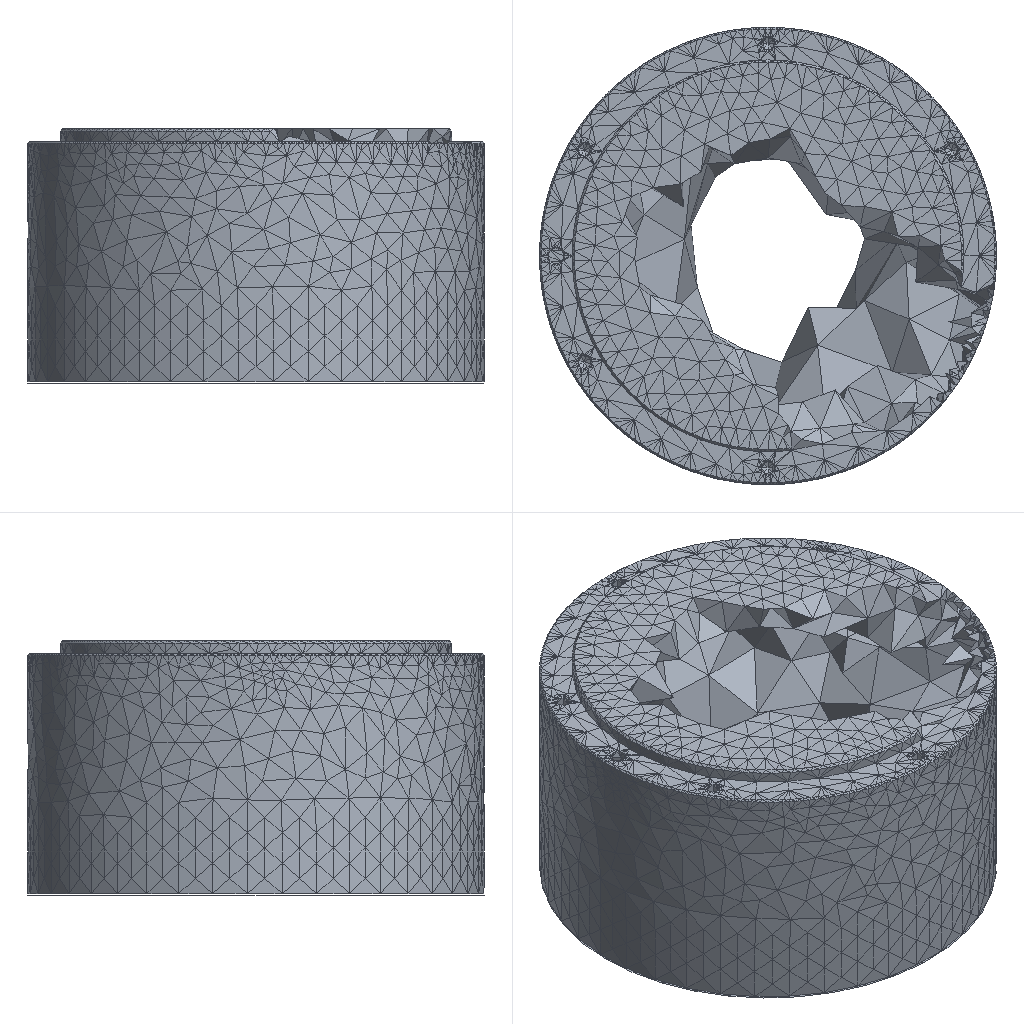Simulation study | ansys workbench
Ansys APDL input file, long lists of numbers shortened:
/batch
/config,noeldb,1     ! force off writing results to database
*get,_wallstrt,active,,time,wall
! ANSYS input file written by Workbench version 2022 R1
/assign,rstp,file,rst              ! Force Eigen analysis to write to file.rst because WB expects it
/solu
antype,,restart,,,perturbation
*DIM,_wb_ProjectScratch_dir_Modal,string,248
_wb_ProjectScratch_dir_Modal(1)= 'C:\_____\_____________\_______\_____\____\________________________\_______________\_______\_
*DIM,_wb_SolverFiles_dir_Modal,string,248
_wb_SolverFiles_dir_Modal(1)= 'C:\_____\_____________\_______\_____\____\________________________\___________\___\_____\____\_
*DIM,_wb_userfiles_dir_Modal,string,248
_wb_userfiles_dir_Modal(1)= 'C:\_____\_____________\_______\_____\____\________________________\___________\__________\_
/title,wbnew--__ (C5)
! ****** Begin Custom Load Command Snippet ******
/COM, ACT Extensions:
/COM,     LSDYNA, 2021.1
/COM,
! ****** End   Custom Load Command Snippet ******
perturb,modal,,CURRENT,DZEROKEEP          ! pre-stress modal analysis, only keep zero bcs in case future MSUP
solve, elform                                       ! Generate matrices needed for perturbation analysis
_thickRatio=  1     ! Ratio of thick parts in the model
modopt,lanb,6
outres,erase
outres,all,none
outres,nsol,all
outres,etmp,all
mxpand                    ! default expand in case of complex solution
dmpopt,esav,no
dmpopt,emat,no
dmpopt,full,no
! *********** WB SOLVE COMMAND ***********
! check interactive state
*get,ANSINTER_,active,,int
*if,ANSINTER_,ne,0,then
/eof
*endif
solve
/com *************** Write FE CONNECTORS *********
CEWRITE,file,ce,,INTE
*get,_nmodalsolproc,active,0,numcpu
fini
/nopr
*get,_numnode,node,0,count
*get,_numelem,elem,0,count
*get, _MAXELEMNUM, elem, 0, NUM, MAX
*get, _MAXNODENUM, node, 0, NUM, MAX,,,INTERNAL
*get, _MAXELEMTYPE, etyp, 0, NUM, MAX
*get, _MAXREALCONST, real, 0, NUM, MAX
/gopr
*get,_wallasol,active,,time,wall
/post1
/nopr
*dim,_direction,CHAR,6,1
_direction(1) = 'X'
_direction(2) = 'Y'
_direction(3) = 'Z'
_direction(4) = 'ROTX'
_direction(5) = 'ROTY'
_direction(6) = 'ROTZ'
*get,_lastLS,active,0,set,LSTP
*get,_beginset,active,0,set,nset,first,_lastLS
*get,_endset,active,0,set,nset,last,_lastLS
_nummodes = 0
*if,_endset,gt,0,then
_nummodes = _endset - _beginset + 1
*endif
*do,i_mode,1,_nummodes
   *do,j_component,1,6
			*get,PFACT_%i_mode%_%j_component%,MODE,%i_mode%,PFACT,,DIREC,_direction(%j_component%)
   *enddo
*enddo
*dim,_tmdirection,CHAR,6,1
_tmdirection(1) = 'X'
_tmdirection(2) = 'Y'
_tmdirection(3) = 'Z'
_tmdirection(4) = 'X'
_tmdirection(5) = 'Y'
_tmdirection(6) = 'Z'
*do,j_component,1,6
    *if,j_component,gt,3,then
        *get,TOTALMASS_%j_component%,ELEM,0,IOR,_tmdirection(%j_component%)
    *else
        *get,TOTALMASS_%j_component%,ELEM,0,MTOT,_tmdirection(%j_component%)
    *endif
*enddo
/gopr
xmlo,ENCODING,ISO-8859-1
xmlo,parm
/xml,parm,xml
fini
/gopr
*get,_walldone,active,,time,wall
_preptime=(_wallbsol-_wallstrt)*3600
_solvtime=(_wallasol-_wallbsol)*3600
_posttime=(_walldone-_wallasol)*3600
_totaltim=(_walldone-_wallstrt)*3600
*get,_dlbratio,active,0,solu,dlbr
*get,_combtime,active,0,solu,comb
*get,_ssmode,active,0,solu,ssmm
*get,_ndofs,active,0,solu,ndof
/fclean				!clean distributed files
/com,--- Total number of nodes = %_numnode%
/com,--- Total number of elements = %_numelem%
/com,--- Element load balance ratio = %_dlbratio%
/com,--- Time to combine distributed files = %_combtime%
/com,--- Sparse memory mode = %_ssmode%
/com,--- Number of DOF = %_ndofs%
/wb,file,end               ! done with WB generated input